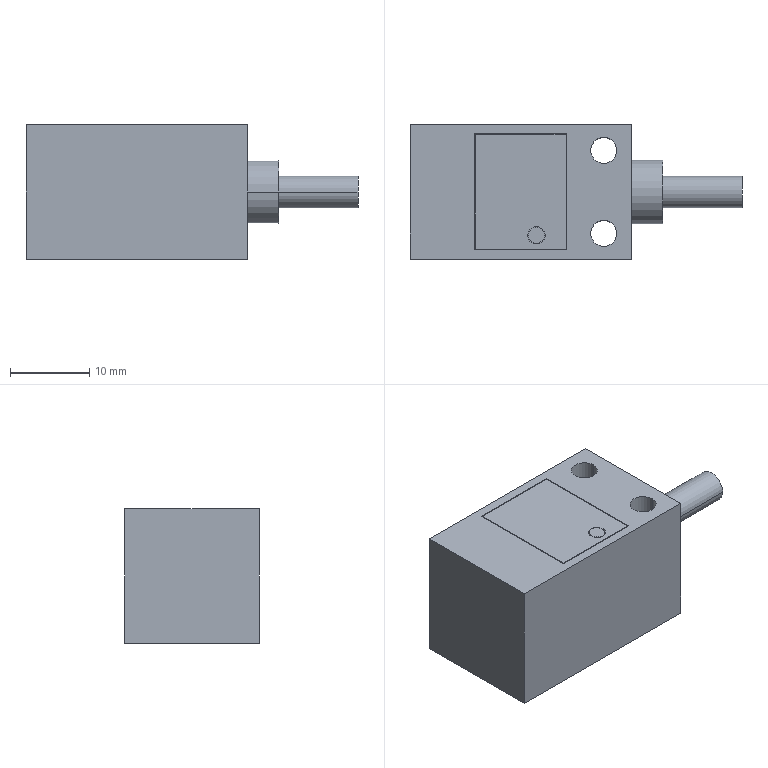Part | SolidWorks | features BaseBody 1 | 1 solid | 65 faces | box 42 x 17 x 17 mm | volume 8111 mm3 | plane 52 | cylinder 13 | commonest cylinder face diameters 3.3 x4 2 x2 2.2 x2 4 x2 8 x2 8.2 x1